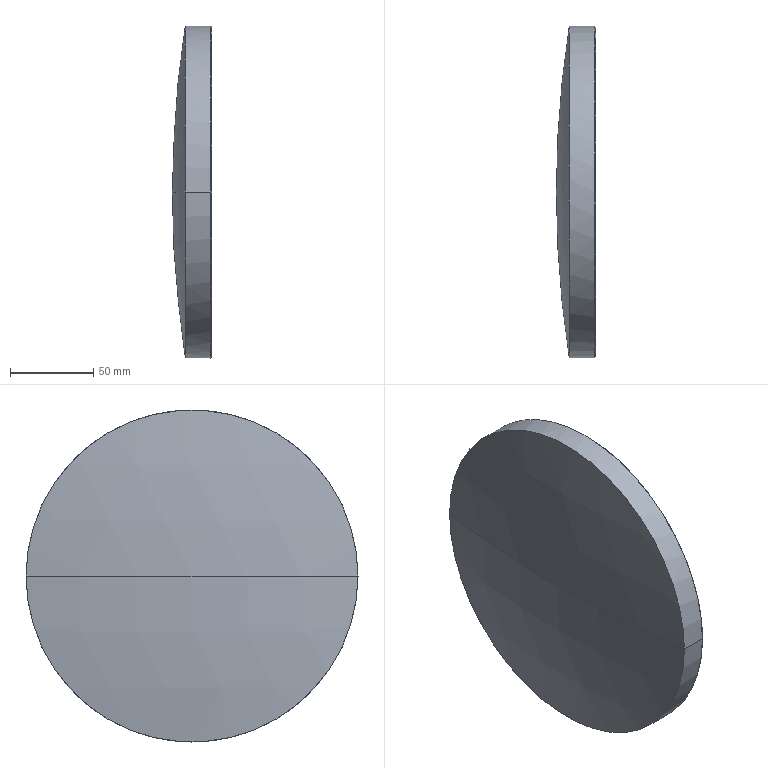Part | STEP file | plano-convex lens 1.stp.STEP-100.STEP | 1 solid | 7 faces | box 23.634 x 200 x 200 mm | volume 620858 mm3 | cylinder 2 | sphere 2 | cone 2 | plane 1 | commonest cylinder face diameters 200 x2
STEP:
#1=CARTESIAN_POINT('',(43.134,0.,-100.));
#2=VERTEX_POINT('',#1);
#3=CARTESIAN_POINT('',(43.134,-100.,0.));
#4=VERTEX_POINT('',#3);
#5=CARTESIAN_POINT('',(43.134,0.,0.));
#6=DIRECTION('',(-1.,0.,0.));
#7=DIRECTION('',(0.,0.,1.));
#8=AXIS2_PLACEMENT_3D('',#5,#6,#7);
#9=CIRCLE('',#8,100.);
#10=EDGE_CURVE('',#2,#4,#9,.T.);
#11=ORIENTED_EDGE('',*,*,#10,.T.);
#12=CARTESIAN_POINT('',(27.754,-100.,0.));
#13=VERTEX_POINT('',#12);
#14=CARTESIAN_POINT('',(0.,-100.,0.));
#15=DIRECTION('',(-1.,0.,0.));
#16=VECTOR('',#15,1000.);
#17=LINE('',#14,#16);
#18=EDGE_CURVE('',#4,#13,#17,.T.);
#19=ORIENTED_EDGE('',*,*,#18,.T.);
#20=CARTESIAN_POINT('',(27.754,100.,0.));
#21=VERTEX_POINT('',#20);
#22=CARTESIAN_POINT('',(27.754,0.,0.));
#23=DIRECTION('',(-1.,0.,0.));
#24=DIRECTION('',(0.,1.,0.));
#25=AXIS2_PLACEMENT_3D('',#22,#23,#24);
#26=CIRCLE('',#25,100.);
#27=EDGE_CURVE('',#21,#13,#26,.T.);
#28=ORIENTED_EDGE('',*,*,#27,.F.);
#29=CARTESIAN_POINT('',(43.134,100.,0.));
#30=VERTEX_POINT('',#29);
#31=CARTESIAN_POINT('',(0.,100.,0.));
#32=DIRECTION('',(-1.,0.,0.));
#33=VECTOR('',#32,1000.);
#34=LINE('',#31,#33);
#35=EDGE_CURVE('',#30,#21,#34,.T.);
#36=ORIENTED_EDGE('',*,*,#35,.F.);
#37=CARTESIAN_POINT('',(43.134,0.,0.));
#38=DIRECTION('',(-1.,0.,0.));
#39=DIRECTION('',(0.,0.,1.));
#40=AXIS2_PLACEMENT_3D('',#37,#38,#39);
#41=CIRCLE('',#40,100.);
#42=EDGE_CURVE('',#30,#2,#41,.T.);
#43=ORIENTED_EDGE('',*,*,#42,.T.);
#44=EDGE_LOOP('',(#11,#19,#28,#36,#43));
#45=FACE_OUTER_BOUND('',#44,.T.);
#46=CARTESIAN_POINT('',(0.,0.,0.));
#47=DIRECTION('',(-1.,0.,0.));
#48=DIRECTION('',(0.,1.,0.));
#49=AXIS2_PLACEMENT_3D('',#46,#47,#48);
#50=CYLINDRICAL_SURFACE('',#49,100.);
#51=ADVANCED_FACE('',(#45),#50,.T.);
#52=ORIENTED_EDGE('',*,*,#27,.T.);
#53=CARTESIAN_POINT('',(668.676,0.,0.));
#54=DIRECTION('',(0.,0.,-1.));
#55=DIRECTION('',(0.,1.,0.));
#56=AXIS2_PLACEMENT_3D('',#53,#54,#55);
#57=CIRCLE('',#56,648.676);
#58=EDGE_CURVE('',#13,#21,#57,.T.);
#59=ORIENTED_EDGE('',*,*,#58,.T.);
#60=EDGE_LOOP('',(#52,#59));
#61=FACE_OUTER_BOUND('',#60,.T.);
#62=CARTESIAN_POINT('',(668.676,0.,0.));
#63=DIRECTION('',(0.,0.,1.));
#64=DIRECTION('',(0.,1.,0.));
#65=AXIS2_PLACEMENT_3D('',#62,#63,#64);
#66=SPHERICAL_SURFACE('',#65,648.676);
#67=ADVANCED_FACE('',(#61),#66,.T.);
#68=CARTESIAN_POINT('',(43.634,0.,-99.5));
#69=VERTEX_POINT('',#68);
#70=CARTESIAN_POINT('',(43.634,0.,99.5));
#71=VERTEX_POINT('',#70);
#72=CARTESIAN_POINT('',(43.634,0.,0.));
#73=DIRECTION('',(1.,0.,0.));
#74=DIRECTION('',(0.,0.,1.));
#75=AXIS2_PLACEMENT_3D('',#72,#73,#74);
#76=CIRCLE('',#75,99.5);
#77=EDGE_CURVE('',#69,#71,#76,.T.);
#78=ORIENTED_EDGE('',*,*,#77,.F.);
#79=CARTESIAN_POINT('',(43.134,0.,-100.));
#80=DIRECTION('',(-0.7071,0.,-0.7071));
#81=VECTOR('',#80,1000.);
#82=LINE('',#79,#81);
#83=EDGE_CURVE('',#69,#2,#82,.T.);
#84=ORIENTED_EDGE('',*,*,#83,.T.);
#85=ORIENTED_EDGE('',*,*,#42,.F.);
#86=CARTESIAN_POINT('',(43.134,0.,100.));
#87=VERTEX_POINT('',#86);
#88=CARTESIAN_POINT('',(43.134,0.,0.));
#89=DIRECTION('',(-1.,0.,0.));
#90=DIRECTION('',(0.,0.,1.));
#91=AXIS2_PLACEMENT_3D('',#88,#89,#90);
#92=CIRCLE('',#91,100.);
#93=EDGE_CURVE('',#87,#30,#92,.T.);
#94=ORIENTED_EDGE('',*,*,#93,.F.);
#95=CARTESIAN_POINT('',(43.134,0.,100.));
#96=DIRECTION('',(-0.7071,0.,0.7071));
#97=VECTOR('',#96,1000.);
#98=LINE('',#95,#97);
#99=EDGE_CURVE('',#71,#87,#98,.T.);
#100=ORIENTED_EDGE('',*,*,#99,.F.);
#101=EDGE_LOOP('',(#78,#84,#85,#94,#100));
#102=FACE_OUTER_BOUND('',#101,.T.);
#103=CARTESIAN_POINT('',(43.134,0.,0.));
#104=DIRECTION('',(-1.,0.,0.));
#105=DIRECTION('',(0.,0.,1.));
#106=AXIS2_PLACEMENT_3D('',#103,#104,#105);
#107=CONICAL_SURFACE('',#106,100.,0.7854);
#108=ADVANCED_FACE('',(#102),#107,.T.);
#109=ORIENTED_EDGE('',*,*,#83,.F.);
#110=CARTESIAN_POINT('',(43.634,0.,0.));
#111=DIRECTION('',(1.,0.,0.));
#112=DIRECTION('',(0.,0.,1.));
#113=AXIS2_PLACEMENT_3D('',#110,#111,#112);
#114=CIRCLE('',#113,99.5);
#115=EDGE_CURVE('',#71,#69,#114,.T.);
#116=ORIENTED_EDGE('',*,*,#115,.F.);
#117=ORIENTED_EDGE('',*,*,#99,.T.);
#118=CARTESIAN_POINT('',(43.134,0.,0.));
#119=DIRECTION('',(-1.,0.,0.));
#120=DIRECTION('',(0.,0.,1.));
#121=AXIS2_PLACEMENT_3D('',#118,#119,#120);
#122=CIRCLE('',#121,100.);
#123=EDGE_CURVE('',#4,#87,#122,.T.);
#124=ORIENTED_EDGE('',*,*,#123,.F.);
#125=ORIENTED_EDGE('',*,*,#10,.F.);
#126=EDGE_LOOP('',(#109,#116,#117,#124,#125));
#127=FACE_OUTER_BOUND('',#126,.T.);
#128=CARTESIAN_POINT('',(43.134,0.,0.));
#129=DIRECTION('',(-1.,0.,0.));
#130=DIRECTION('',(0.,0.,1.));
#131=AXIS2_PLACEMENT_3D('',#128,#129,#130);
#132=CONICAL_SURFACE('',#131,100.,0.7854);
#133=ADVANCED_FACE('',(#127),#132,.T.);
#134=ORIENTED_EDGE('',*,*,#58,.F.);
#135=CARTESIAN_POINT('',(27.754,0.,0.));
#136=DIRECTION('',(-1.,0.,0.));
#137=DIRECTION('',(0.,1.,0.));
#138=AXIS2_PLACEMENT_3D('',#135,#136,#137);
#139=CIRCLE('',#138,100.);
#140=EDGE_CURVE('',#13,#21,#139,.T.);
#141=ORIENTED_EDGE('',*,*,#140,.T.);
#142=EDGE_LOOP('',(#134,#141));
#143=FACE_OUTER_BOUND('',#142,.T.);
#144=CARTESIAN_POINT('',(668.676,0.,0.));
#145=DIRECTION('',(0.,0.,1.));
#146=DIRECTION('',(0.,1.,0.));
#147=AXIS2_PLACEMENT_3D('',#144,#145,#146);
#148=SPHERICAL_SURFACE('',#147,648.676);
#149=ADVANCED_FACE('',(#143),#148,.T.);
#150=ORIENTED_EDGE('',*,*,#18,.F.);
#151=ORIENTED_EDGE('',*,*,#123,.T.);
#152=ORIENTED_EDGE('',*,*,#93,.T.);
#153=ORIENTED_EDGE('',*,*,#35,.T.);
#154=ORIENTED_EDGE('',*,*,#140,.F.);
#155=EDGE_LOOP('',(#150,#151,#152,#153,#154));
#156=FACE_OUTER_BOUND('',#155,.T.);
#157=CARTESIAN_POINT('',(0.,0.,0.));
#158=DIRECTION('',(-1.,0.,0.));
#159=DIRECTION('',(0.,1.,0.));
#160=AXIS2_PLACEMENT_3D('',#157,#158,#159);
#161=CYLINDRICAL_SURFACE('',#160,100.);
#162=ADVANCED_FACE('',(#156),#161,.T.);
#163=ORIENTED_EDGE('',*,*,#115,.T.);
#164=ORIENTED_EDGE('',*,*,#77,.T.);
#165=EDGE_LOOP('',(#163,#164));
#166=FACE_OUTER_BOUND('',#165,.T.);
#167=CARTESIAN_POINT('',(43.634,0.,0.));
#168=DIRECTION('',(-1.,0.,0.));
#169=DIRECTION('',(0.,0.,1.));
#170=AXIS2_PLACEMENT_3D('',#167,#168,#169);
#171=PLANE('',#170);
#172=ADVANCED_FACE('',(#166),#171,.F.);
#173=CLOSED_SHELL('',(#51,#67,#108,#133,#149,#162,#172));
#174=MANIFOLD_SOLID_BREP('',#173);
#175=CARTESIAN_POINT('',(0.,0.,0.));
#176=DIRECTION('',(0.,0.,1.));
#177=DIRECTION('',(1.,0.,0.));
#178=AXIS2_PLACEMENT_3D('',#175,#176,#177);
#179=(LENGTH_UNIT()NAMED_UNIT(*)SI_UNIT(.MILLI.,.METRE.));
#180=UNCERTAINTY_MEASURE_WITH_UNIT(LENGTH_MEASURE(0.00001),#179,'','');
#181=(NAMED_UNIT(*)PLANE_ANGLE_UNIT()SI_UNIT($,.RADIAN.));
#182=(NAMED_UNIT(*)SI_UNIT($,.STERADIAN.)SOLID_ANGLE_UNIT());
#183=(GEOMETRIC_REPRESENTATION_CONTEXT(3)GLOBAL_UNCERTAINTY_ASSIGNED_CONTEXT((#180))GLOBAL_UNIT_ASSIGNED_CONTEXT((#179,#181,#182))REPRESENTATION_CONTEXT('',''));
#184=ADVANCED_BREP_SHAPE_REPRESENTATION('',(#174,#178),#183);